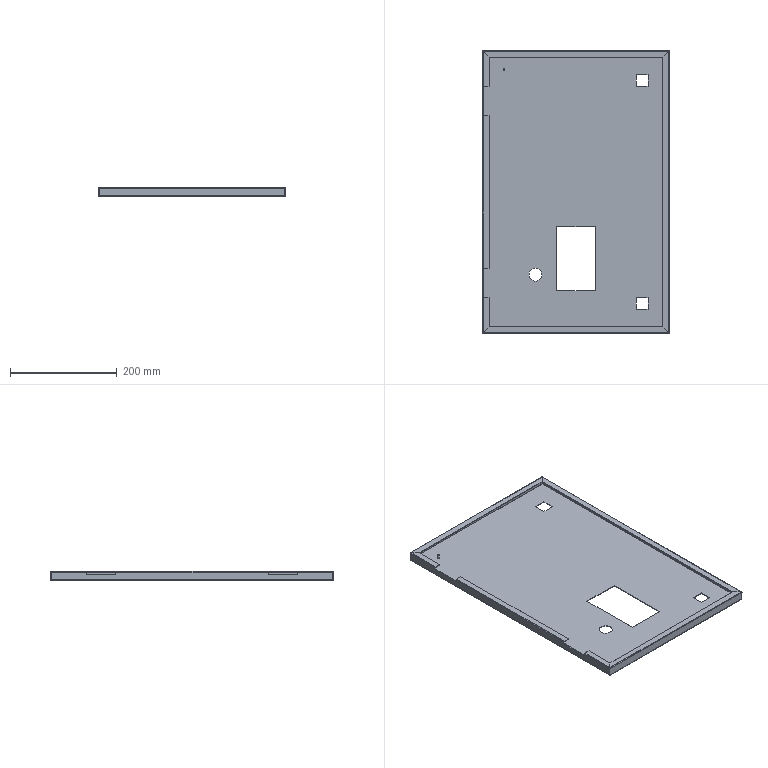Part | STEP file | 1 solid | 123 faces | box 350 x 530 x 17 mm | volume 262811 mm3 | plane 87 | cylinder 24 | spline 12 | commonest cylinder face diameters 0.02 x10 2.42 x10 3 x2 24 x2